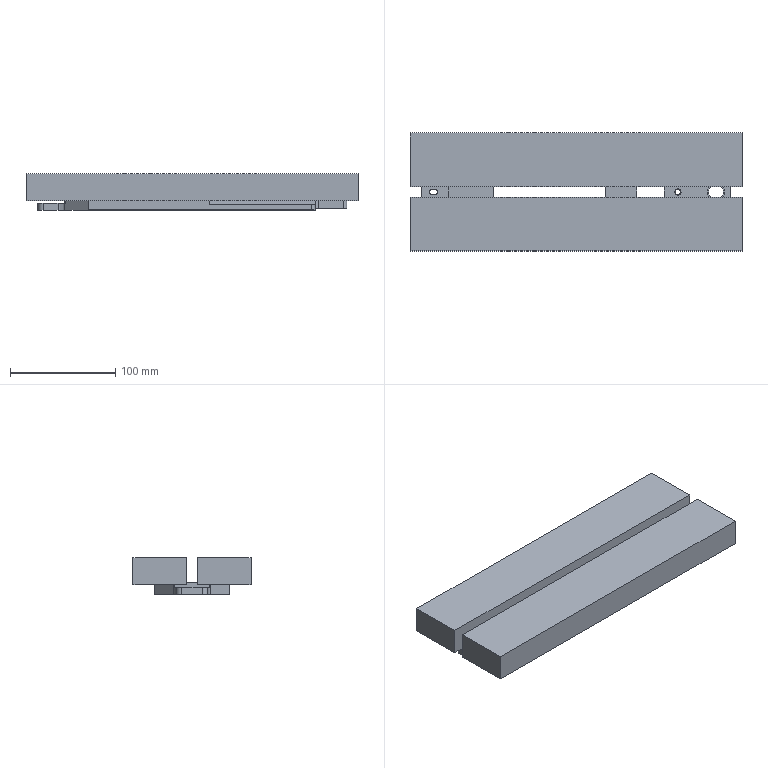Part | 3 solids | 199 faces | box 315 x 112 x 34.85 mm | volume 893092 mm3 | plane 99 | cylinder 80 | cone 20 | commonest cylinder face diameters 3.4 x16 6 x12 10 x9 2.05 x8 4 x8 20 x6